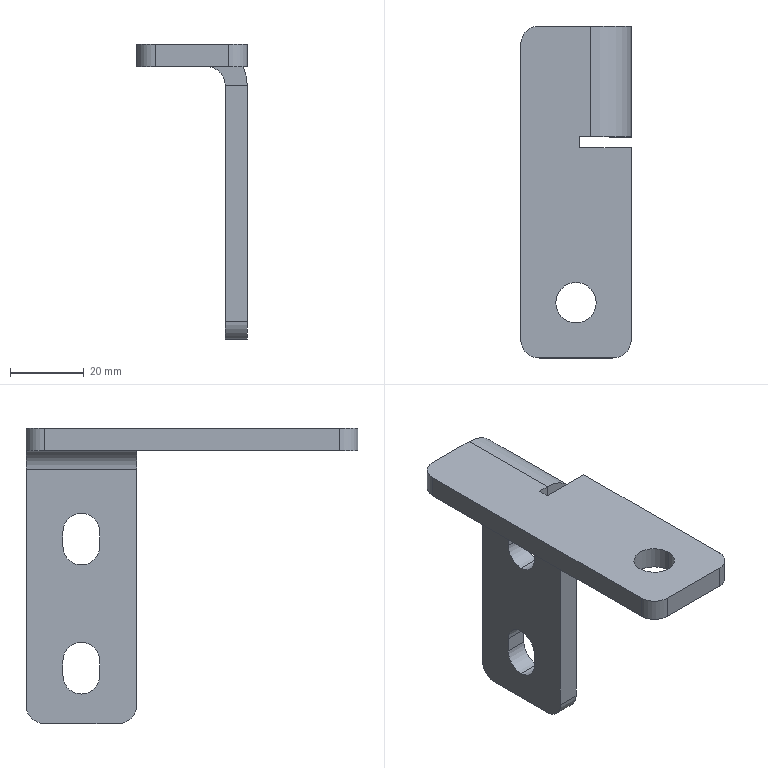Part | STEP file | SYL_0392D6J1SYL0380DJ1006_2_6-5 | 1 solid | 37 faces | box 30 x 90 x 80 mm | volume 26496 mm3 | plane 20 | cylinder 17 | commonest cylinder face diameters 10 x14 11 x2 22 x1
STEP:
#1=CARTESIAN_POINT('',(15.,35.,-61.));
#2=VERTEX_POINT('',#1);
#3=CARTESIAN_POINT('',(9.,35.,-61.));
#4=VERTEX_POINT('',#3);
#5=CARTESIAN_POINT('',(9.,35.,-61.));
#6=DIRECTION('',(-1.,0.,0.));
#7=VECTOR('',#6,1000.);
#8=LINE('',#5,#7);
#9=EDGE_CURVE('',#2,#4,#8,.T.);
#10=ORIENTED_EDGE('',*,*,#9,.F.);
#11=CARTESIAN_POINT('',(15.,35.,-57.));
#12=VERTEX_POINT('',#11);
#13=CARTESIAN_POINT('',(15.,35.,6.));
#14=DIRECTION('',(0.,0.,1.));
#15=VECTOR('',#14,1000.);
#16=LINE('',#13,#15);
#17=EDGE_CURVE('',#2,#12,#16,.T.);
#18=ORIENTED_EDGE('',*,*,#17,.T.);
#19=CARTESIAN_POINT('',(9.,35.,-57.));
#20=VERTEX_POINT('',#19);
#21=CARTESIAN_POINT('',(9.,35.,-57.));
#22=DIRECTION('',(-1.,0.,0.));
#23=VECTOR('',#22,1000.);
#24=LINE('',#21,#23);
#25=EDGE_CURVE('',#12,#20,#24,.T.);
#26=ORIENTED_EDGE('',*,*,#25,.T.);
#27=CARTESIAN_POINT('',(9.,35.,-61.));
#28=DIRECTION('',(0.,0.,1.));
#29=VECTOR('',#28,1000.);
#30=LINE('',#27,#29);
#31=EDGE_CURVE('',#4,#20,#30,.T.);
#32=ORIENTED_EDGE('',*,*,#31,.F.);
#33=EDGE_LOOP('',(#10,#18,#26,#32));
#34=FACE_OUTER_BOUND('',#33,.T.);
#35=CARTESIAN_POINT('',(9.,35.,-61.));
#36=DIRECTION('',(0.,1.,0.));
#37=DIRECTION('',(0.,0.,1.));
#38=AXIS2_PLACEMENT_3D('',#35,#36,#37);
#39=PLANE('',#38);
#40=ADVANCED_FACE('',(#34),#39,.F.);
#41=ORIENTED_EDGE('',*,*,#25,.F.);
#42=CARTESIAN_POINT('',(15.,30.,-52.));
#43=VERTEX_POINT('',#42);
#44=CARTESIAN_POINT('',(15.,30.,-57.));
#45=DIRECTION('',(1.,0.,0.));
#46=DIRECTION('',(0.,0.,-1.));
#47=AXIS2_PLACEMENT_3D('',#44,#45,#46);
#48=CIRCLE('',#47,5.);
#49=EDGE_CURVE('',#12,#43,#48,.T.);
#50=ORIENTED_EDGE('',*,*,#49,.T.);
#51=CARTESIAN_POINT('',(9.,30.,-52.));
#52=VERTEX_POINT('',#51);
#53=CARTESIAN_POINT('',(9.,30.,-52.));
#54=DIRECTION('',(-1.,0.,0.));
#55=VECTOR('',#54,1000.);
#56=LINE('',#53,#55);
#57=EDGE_CURVE('',#43,#52,#56,.T.);
#58=ORIENTED_EDGE('',*,*,#57,.T.);
#59=CARTESIAN_POINT('',(9.,30.,-57.));
#60=DIRECTION('',(1.,0.,0.));
#61=DIRECTION('',(0.,1.,0.));
#62=AXIS2_PLACEMENT_3D('',#59,#60,#61);
#63=CIRCLE('',#62,5.);
#64=EDGE_CURVE('',#20,#52,#63,.T.);
#65=ORIENTED_EDGE('',*,*,#64,.F.);
#66=EDGE_LOOP('',(#41,#50,#58,#65));
#67=FACE_OUTER_BOUND('',#66,.T.);
#68=CARTESIAN_POINT('',(9.,30.,-57.));
#69=DIRECTION('',(1.,0.,0.));
#70=DIRECTION('',(0.,0.,-1.));
#71=AXIS2_PLACEMENT_3D('',#68,#69,#70);
#72=CYLINDRICAL_SURFACE('',#71,5.);
#73=ADVANCED_FACE('',(#67),#72,.F.);
#74=ORIENTED_EDGE('',*,*,#57,.F.);
#75=CARTESIAN_POINT('',(15.,25.,-57.));
#76=VERTEX_POINT('',#75);
#77=CARTESIAN_POINT('',(15.,30.,-57.));
#78=DIRECTION('',(1.,0.,0.));
#79=DIRECTION('',(0.,0.,-1.));
#80=AXIS2_PLACEMENT_3D('',#77,#78,#79);
#81=CIRCLE('',#80,5.);
#82=EDGE_CURVE('',#43,#76,#81,.T.);
#83=ORIENTED_EDGE('',*,*,#82,.T.);
#84=CARTESIAN_POINT('',(9.,25.,-57.));
#85=VERTEX_POINT('',#84);
#86=CARTESIAN_POINT('',(9.,25.,-57.));
#87=DIRECTION('',(-1.,0.,0.));
#88=VECTOR('',#87,1000.);
#89=LINE('',#86,#88);
#90=EDGE_CURVE('',#76,#85,#89,.T.);
#91=ORIENTED_EDGE('',*,*,#90,.T.);
#92=CARTESIAN_POINT('',(9.,30.,-57.));
#93=DIRECTION('',(1.,0.,0.));
#94=DIRECTION('',(0.,0.,1.));
#95=AXIS2_PLACEMENT_3D('',#92,#93,#94);
#96=CIRCLE('',#95,5.);
#97=EDGE_CURVE('',#52,#85,#96,.T.);
#98=ORIENTED_EDGE('',*,*,#97,.F.);
#99=EDGE_LOOP('',(#74,#83,#91,#98));
#100=FACE_OUTER_BOUND('',#99,.T.);
#101=CARTESIAN_POINT('',(9.,30.,-57.));
#102=DIRECTION('',(1.,0.,0.));
#103=DIRECTION('',(0.,0.,-1.));
#104=AXIS2_PLACEMENT_3D('',#101,#102,#103);
#105=CYLINDRICAL_SURFACE('',#104,5.);
#106=ADVANCED_FACE('',(#100),#105,.F.);
#107=ORIENTED_EDGE('',*,*,#90,.F.);
#108=CARTESIAN_POINT('',(15.,25.,-61.));
#109=VERTEX_POINT('',#108);
#110=CARTESIAN_POINT('',(15.,25.,6.));
#111=DIRECTION('',(0.,0.,-1.));
#112=VECTOR('',#111,1000.);
#113=LINE('',#110,#112);
#114=EDGE_CURVE('',#76,#109,#113,.T.);
#115=ORIENTED_EDGE('',*,*,#114,.T.);
#116=CARTESIAN_POINT('',(9.,25.,-61.));
#117=VERTEX_POINT('',#116);
#118=CARTESIAN_POINT('',(9.,25.,-61.));
#119=DIRECTION('',(-1.,0.,0.));
#120=VECTOR('',#119,1000.);
#121=LINE('',#118,#120);
#122=EDGE_CURVE('',#109,#117,#121,.T.);
#123=ORIENTED_EDGE('',*,*,#122,.T.);
#124=CARTESIAN_POINT('',(9.,25.,-57.));
#125=DIRECTION('',(0.,0.,-1.));
#126=VECTOR('',#125,1000.);
#127=LINE('',#124,#126);
#128=EDGE_CURVE('',#85,#117,#127,.T.);
#129=ORIENTED_EDGE('',*,*,#128,.F.);
#130=EDGE_LOOP('',(#107,#115,#123,#129));
#131=FACE_OUTER_BOUND('',#130,.T.);
#132=CARTESIAN_POINT('',(9.,25.,-57.));
#133=DIRECTION('',(0.,-1.,0.));
#134=DIRECTION('',(0.,0.,-1.));
#135=AXIS2_PLACEMENT_3D('',#132,#133,#134);
#136=PLANE('',#135);
#137=ADVANCED_FACE('',(#131),#136,.F.);
#138=ORIENTED_EDGE('',*,*,#122,.F.);
#139=CARTESIAN_POINT('',(15.,30.,-66.));
#140=VERTEX_POINT('',#139);
#141=CARTESIAN_POINT('',(15.,30.,-61.));
#142=DIRECTION('',(1.,0.,0.));
#143=DIRECTION('',(0.,0.,-1.));
#144=AXIS2_PLACEMENT_3D('',#141,#142,#143);
#145=CIRCLE('',#144,5.);
#146=EDGE_CURVE('',#109,#140,#145,.T.);
#147=ORIENTED_EDGE('',*,*,#146,.T.);
#148=CARTESIAN_POINT('',(9.,30.,-66.));
#149=VERTEX_POINT('',#148);
#150=CARTESIAN_POINT('',(9.,30.,-66.));
#151=DIRECTION('',(-1.,0.,0.));
#152=VECTOR('',#151,1000.);
#153=LINE('',#150,#152);
#154=EDGE_CURVE('',#140,#149,#153,.T.);
#155=ORIENTED_EDGE('',*,*,#154,.T.);
#156=CARTESIAN_POINT('',(9.,30.,-61.));
#157=DIRECTION('',(1.,0.,0.));
#158=DIRECTION('',(0.,-1.,0.));
#159=AXIS2_PLACEMENT_3D('',#156,#157,#158);
#160=CIRCLE('',#159,5.);
#161=EDGE_CURVE('',#117,#149,#160,.T.);
#162=ORIENTED_EDGE('',*,*,#161,.F.);
#163=EDGE_LOOP('',(#138,#147,#155,#162));
#164=FACE_OUTER_BOUND('',#163,.T.);
#165=CARTESIAN_POINT('',(9.,30.,-61.));
#166=DIRECTION('',(1.,0.,0.));
#167=DIRECTION('',(0.,0.,-1.));
#168=AXIS2_PLACEMENT_3D('',#165,#166,#167);
#169=CYLINDRICAL_SURFACE('',#168,5.);
#170=ADVANCED_FACE('',(#164),#169,.F.);
#171=CARTESIAN_POINT('',(15.,35.,-26.));
#172=VERTEX_POINT('',#171);
#173=CARTESIAN_POINT('',(9.,35.,-26.));
#174=VERTEX_POINT('',#173);
#175=CARTESIAN_POINT('',(9.,35.,-26.));
#176=DIRECTION('',(-1.,0.,0.));
#177=VECTOR('',#176,1000.);
#178=LINE('',#175,#177);
#179=EDGE_CURVE('',#172,#174,#178,.T.);
#180=ORIENTED_EDGE('',*,*,#179,.F.);
#181=CARTESIAN_POINT('',(15.,35.,-22.));
#182=VERTEX_POINT('',#181);
#183=CARTESIAN_POINT('',(15.,35.,6.));
#184=DIRECTION('',(0.,0.,1.));
#185=VECTOR('',#184,1000.);
#186=LINE('',#183,#185);
#187=EDGE_CURVE('',#172,#182,#186,.T.);
#188=ORIENTED_EDGE('',*,*,#187,.T.);
#189=CARTESIAN_POINT('',(9.,35.,-22.));
#190=VERTEX_POINT('',#189);
#191=CARTESIAN_POINT('',(9.,35.,-22.));
#192=DIRECTION('',(-1.,0.,0.));
#193=VECTOR('',#192,1000.);
#194=LINE('',#191,#193);
#195=EDGE_CURVE('',#182,#190,#194,.T.);
#196=ORIENTED_EDGE('',*,*,#195,.T.);
#197=CARTESIAN_POINT('',(9.,35.,-26.));
#198=DIRECTION('',(0.,0.,1.));
#199=VECTOR('',#198,1000.);
#200=LINE('',#197,#199);
#201=EDGE_CURVE('',#174,#190,#200,.T.);
#202=ORIENTED_EDGE('',*,*,#201,.F.);
#203=EDGE_LOOP('',(#180,#188,#196,#202));
#204=FACE_OUTER_BOUND('',#203,.T.);
#205=CARTESIAN_POINT('',(9.,35.,-26.));
#206=DIRECTION('',(0.,1.,0.));
#207=DIRECTION('',(0.,0.,1.));
#208=AXIS2_PLACEMENT_3D('',#205,#206,#207);
#209=PLANE('',#208);
#210=ADVANCED_FACE('',(#204),#209,.F.);
#211=ORIENTED_EDGE('',*,*,#195,.F.);
#212=CARTESIAN_POINT('',(15.,30.,-17.));
#213=VERTEX_POINT('',#212);
#214=CARTESIAN_POINT('',(15.,30.,-22.));
#215=DIRECTION('',(1.,0.,0.));
#216=DIRECTION('',(0.,0.,-1.));
#217=AXIS2_PLACEMENT_3D('',#214,#215,#216);
#218=CIRCLE('',#217,5.);
#219=EDGE_CURVE('',#182,#213,#218,.T.);
#220=ORIENTED_EDGE('',*,*,#219,.T.);
#221=CARTESIAN_POINT('',(9.,30.,-17.));
#222=VERTEX_POINT('',#221);
#223=CARTESIAN_POINT('',(9.,30.,-17.));
#224=DIRECTION('',(-1.,0.,0.));
#225=VECTOR('',#224,1000.);
#226=LINE('',#223,#225);
#227=EDGE_CURVE('',#213,#222,#226,.T.);
#228=ORIENTED_EDGE('',*,*,#227,.T.);
#229=CARTESIAN_POINT('',(9.,30.,-22.));
#230=DIRECTION('',(1.,0.,0.));
#231=DIRECTION('',(0.,1.,0.));
#232=AXIS2_PLACEMENT_3D('',#229,#230,#231);
#233=CIRCLE('',#232,5.);
#234=EDGE_CURVE('',#190,#222,#233,.T.);
#235=ORIENTED_EDGE('',*,*,#234,.F.);
#236=EDGE_LOOP('',(#211,#220,#228,#235));
#237=FACE_OUTER_BOUND('',#236,.T.);
#238=CARTESIAN_POINT('',(9.,30.,-22.));
#239=DIRECTION('',(1.,0.,0.));
#240=DIRECTION('',(0.,0.,-1.));
#241=AXIS2_PLACEMENT_3D('',#238,#239,#240);
#242=CYLINDRICAL_SURFACE('',#241,5.);
#243=ADVANCED_FACE('',(#237),#242,.F.);
#244=ORIENTED_EDGE('',*,*,#227,.F.);
#245=CARTESIAN_POINT('',(15.,25.,-22.));
#246=VERTEX_POINT('',#245);
#247=CARTESIAN_POINT('',(15.,30.,-22.));
#248=DIRECTION('',(1.,0.,0.));
#249=DIRECTION('',(0.,0.,-1.));
#250=AXIS2_PLACEMENT_3D('',#247,#248,#249);
#251=CIRCLE('',#250,5.);
#252=EDGE_CURVE('',#213,#246,#251,.T.);
#253=ORIENTED_EDGE('',*,*,#252,.T.);
#254=CARTESIAN_POINT('',(9.,25.,-22.));
#255=VERTEX_POINT('',#254);
#256=CARTESIAN_POINT('',(9.,25.,-22.));
#257=DIRECTION('',(-1.,0.,0.));
#258=VECTOR('',#257,1000.);
#259=LINE('',#256,#258);
#260=EDGE_CURVE('',#246,#255,#259,.T.);
#261=ORIENTED_EDGE('',*,*,#260,.T.);
#262=CARTESIAN_POINT('',(9.,30.,-22.));
#263=DIRECTION('',(1.,0.,0.));
#264=DIRECTION('',(0.,0.,1.));
#265=AXIS2_PLACEMENT_3D('',#262,#263,#264);
#266=CIRCLE('',#265,5.);
#267=EDGE_CURVE('',#222,#255,#266,.T.);
#268=ORIENTED_EDGE('',*,*,#267,.F.);
#269=EDGE_LOOP('',(#244,#253,#261,#268));
#270=FACE_OUTER_BOUND('',#269,.T.);
#271=CARTESIAN_POINT('',(9.,30.,-22.));
#272=DIRECTION('',(1.,0.,0.));
#273=DIRECTION('',(0.,0.,-1.));
#274=AXIS2_PLACEMENT_3D('',#271,#272,#273);
#275=CYLINDRICAL_SURFACE('',#274,5.);
#276=ADVANCED_FACE('',(#270),#275,.F.);
#277=ORIENTED_EDGE('',*,*,#260,.F.);
#278=CARTESIAN_POINT('',(15.,25.,-26.));
#279=VERTEX_POINT('',#278);
#280=CARTESIAN_POINT('',(15.,25.,6.));
#281=DIRECTION('',(0.,0.,-1.));
#282=VECTOR('',#281,1000.);
#283=LINE('',#280,#282);
#284=EDGE_CURVE('',#246,#279,#283,.T.);
#285=ORIENTED_EDGE('',*,*,#284,.T.);
#286=CARTESIAN_POINT('',(9.,25.,-26.));
#287=VERTEX_POINT('',#286);
#288=CARTESIAN_POINT('',(9.,25.,-26.));
#289=DIRECTION('',(-1.,0.,0.));
#290=VECTOR('',#289,1000.);
#291=LINE('',#288,#290);
#292=EDGE_CURVE('',#279,#287,#291,.T.);
#293=ORIENTED_EDGE('',*,*,#292,.T.);
#294=CARTESIAN_POINT('',(9.,25.,-22.));
#295=DIRECTION('',(0.,0.,-1.));
#296=VECTOR('',#295,1000.);
#297=LINE('',#294,#296);
#298=EDGE_CURVE('',#255,#287,#297,.T.);
#299=ORIENTED_EDGE('',*,*,#298,.F.);
#300=EDGE_LOOP('',(#277,#285,#293,#299));
#301=FACE_OUTER_BOUND('',#300,.T.);
#302=CARTESIAN_POINT('',(9.,25.,-22.));
#303=DIRECTION('',(0.,-1.,0.));
#304=DIRECTION('',(0.,0.,-1.));
#305=AXIS2_PLACEMENT_3D('',#302,#303,#304);
#306=PLANE('',#305);
#307=ADVANCED_FACE('',(#301),#306,.F.);
#308=ORIENTED_EDGE('',*,*,#292,.F.);
#309=CARTESIAN_POINT('',(15.,30.,-31.));
#310=VERTEX_POINT('',#309);
#311=CARTESIAN_POINT('',(15.,30.,-26.));
#312=DIRECTION('',(1.,0.,0.));
#313=DIRECTION('',(0.,0.,-1.));
#314=AXIS2_PLACEMENT_3D('',#311,#312,#313);
#315=CIRCLE('',#314,5.);
#316=EDGE_CURVE('',#279,#310,#315,.T.);
#317=ORIENTED_EDGE('',*,*,#316,.T.);
#318=CARTESIAN_POINT('',(9.,30.,-31.));
#319=VERTEX_POINT('',#318);
#320=CARTESIAN_POINT('',(9.,30.,-31.));
#321=DIRECTION('',(-1.,0.,0.));
#322=VECTOR('',#321,1000.);
#323=LINE('',#320,#322);
#324=EDGE_CURVE('',#310,#319,#323,.T.);
#325=ORIENTED_EDGE('',*,*,#324,.T.);
#326=CARTESIAN_POINT('',(9.,30.,-26.));
#327=DIRECTION('',(1.,0.,0.));
#328=DIRECTION('',(0.,-1.,0.));
#329=AXIS2_PLACEMENT_3D('',#326,#327,#328);
#330=CIRCLE('',#329,5.);
#331=EDGE_CURVE('',#287,#319,#330,.T.);
#332=ORIENTED_EDGE('',*,*,#331,.F.);
#333=EDGE_LOOP('',(#308,#317,#325,#332));
#334=FACE_OUTER_BOUND('',#333,.T.);
#335=CARTESIAN_POINT('',(9.,30.,-26.));
#336=DIRECTION('',(1.,0.,0.));
#337=DIRECTION('',(0.,0.,-1.));
#338=AXIS2_PLACEMENT_3D('',#335,#336,#337);
#339=CYLINDRICAL_SURFACE('',#338,5.);
#340=ADVANCED_FACE('',(#334),#339,.F.);
#341=CARTESIAN_POINT('',(-5.5,-30.,6.));
#342=VERTEX_POINT('',#341);
#343=CARTESIAN_POINT('',(-5.5,-30.,0.));
#344=VERTEX_POINT('',#343);
#345=CARTESIAN_POINT('',(-5.5,-30.,0.));
#346=DIRECTION('',(0.,0.,-1.));
#347=VECTOR('',#346,1000.);
#348=LINE('',#345,#347);
#349=EDGE_CURVE('',#342,#344,#348,.T.);
#350=ORIENTED_EDGE('',*,*,#349,.F.);
#351=CARTESIAN_POINT('',(5.5,-30.,6.));
#352=VERTEX_POINT('',#351);
#353=CARTESIAN_POINT('',(0.,-30.,6.));
#354=DIRECTION('',(0.,0.,1.));
#355=DIRECTION('',(1.,0.,0.));
#356=AXIS2_PLACEMENT_3D('',#353,#354,#355);
#357=CIRCLE('',#356,5.5);
#358=EDGE_CURVE('',#342,#352,#357,.T.);
#359=ORIENTED_EDGE('',*,*,#358,.T.);
#360=CARTESIAN_POINT('',(5.5,-30.,0.));
#361=VERTEX_POINT('',#360);
#362=CARTESIAN_POINT('',(5.5,-30.,0.));
#363=DIRECTION('',(0.,0.,-1.));
#364=VECTOR('',#363,1000.);
#365=LINE('',#362,#364);
#366=EDGE_CURVE('',#352,#361,#365,.T.);
#367=ORIENTED_EDGE('',*,*,#366,.T.);
#368=CARTESIAN_POINT('',(0.,-30.,0.));
#369=DIRECTION('',(0.,0.,1.));
#370=DIRECTION('',(-1.,0.,0.));
#371=AXIS2_PLACEMENT_3D('',#368,#369,#370);
#372=CIRCLE('',#371,5.5);
#373=EDGE_CURVE('',#344,#361,#372,.T.);
#374=ORIENTED_EDGE('',*,*,#373,.F.);
#375=EDGE_LOOP('',(#350,#359,#367,#374));
#376=FACE_OUTER_BOUND('',#375,.T.);
#377=CARTESIAN_POINT('',(0.,-30.,0.));
#378=DIRECTION('',(0.,0.,1.));
#379=DIRECTION('',(1.,0.,0.));
#380=AXIS2_PLACEMENT_3D('',#377,#378,#379);
#381=CYLINDRICAL_SURFACE('',#380,5.5);
#382=ADVANCED_FACE('',(#376),#381,.F.);
#383=CARTESIAN_POINT('',(15.,45.,-69.));
#384=VERTEX_POINT('',#383);
#385=CARTESIAN_POINT('',(9.,45.,-69.));
#386=VERTEX_POINT('',#385);
#387=CARTESIAN_POINT('',(9.,45.,-69.));
#388=DIRECTION('',(-1.,0.,0.));
#389=VECTOR('',#388,1000.);
#390=LINE('',#387,#389);
#391=EDGE_CURVE('',#384,#386,#390,.T.);
#392=ORIENTED_EDGE('',*,*,#391,.F.);
#393=CARTESIAN_POINT('',(15.,40.,-74.));
#394=VERTEX_POINT('',#393);
#395=CARTESIAN_POINT('',(15.,40.,-69.));
#396=DIRECTION('',(-1.,0.,0.));
#397=DIRECTION('',(0.,0.,1.));
#398=AXIS2_PLACEMENT_3D('',#395,#396,#397);
#399=CIRCLE('',#398,5.);
#400=EDGE_CURVE('',#384,#394,#399,.T.);
#401=ORIENTED_EDGE('',*,*,#400,.T.);
#402=CARTESIAN_POINT('',(9.,40.,-74.));
#403=VERTEX_POINT('',#402);
#404=CARTESIAN_POINT('',(9.,40.,-74.));
#405=DIRECTION('',(-1.,0.,0.));
#406=VECTOR('',#405,1000.);
#407=LINE('',#404,#406);
#408=EDGE_CURVE('',#394,#403,#407,.T.);
#409=ORIENTED_EDGE('',*,*,#408,.T.);
#410=CARTESIAN_POINT('',(9.,40.,-69.));
#411=DIRECTION('',(-1.,0.,0.));
#412=DIRECTION('',(0.,1.,0.));
#413=AXIS2_PLACEMENT_3D('',#410,#411,#412);
#414=CIRCLE('',#413,5.);
#415=EDGE_CURVE('',#386,#403,#414,.T.);
#416=ORIENTED_EDGE('',*,*,#415,.F.);
#417=EDGE_LOOP('',(#392,#401,#409,#416));
#418=FACE_OUTER_BOUND('',#417,.T.);
#419=CARTESIAN_POINT('',(9.,40.,-69.));
#420=DIRECTION('',(1.,0.,0.));
#421=DIRECTION('',(0.,0.,-1.));
#422=AXIS2_PLACEMENT_3D('',#419,#420,#421);
#423=CYLINDRICAL_SURFACE('',#422,5.);
#424=ADVANCED_FACE('',(#418),#423,.T.);
#425=ORIENTED_EDGE('',*,*,#408,.F.);
#426=CARTESIAN_POINT('',(15.,20.,-74.));
#427=VERTEX_POINT('',#426);
#428=CARTESIAN_POINT('',(15.,-23.616,-74.));
#429=DIRECTION('',(0.,-1.,0.));
#430=VECTOR('',#429,1000.);
#431=LINE('',#428,#430);
#432=EDGE_CURVE('',#394,#427,#431,.T.);
#433=ORIENTED_EDGE('',*,*,#432,.T.);
#434=CARTESIAN_POINT('',(9.,20.,-74.));
#435=VERTEX_POINT('',#434);
#436=CARTESIAN_POINT('',(9.,20.,-74.));
#437=DIRECTION('',(-1.,0.,0.));
#438=VECTOR('',#437,1000.);
#439=LINE('',#436,#438);
#440=EDGE_CURVE('',#427,#435,#439,.T.);
#441=ORIENTED_EDGE('',*,*,#440,.T.);
#442=CARTESIAN_POINT('',(9.,40.,-74.));
#443=DIRECTION('',(0.,-1.,0.));
#444=VECTOR('',#443,1000.);
#445=LINE('',#442,#444);
#446=EDGE_CURVE('',#403,#435,#445,.T.);
#447=ORIENTED_EDGE('',*,*,#446,.F.);
#448=EDGE_LOOP('',(#425,#433,#441,#447));
#449=FACE_OUTER_BOUND('',#448,.T.);
#450=CARTESIAN_POINT('',(9.,40.,-74.));
#451=DIRECTION('',(0.,0.,1.));
#452=DIRECTION('',(0.,-1.,0.));
#453=AXIS2_PLACEMENT_3D('',#450,#451,#452);
#454=PLANE('',#453);
#455=ADVANCED_FACE('',(#449),#454,.F.);
#456=ORIENTED_EDGE('',*,*,#440,.F.);
#457=CARTESIAN_POINT('',(15.,15.,-69.));
#458=VERTEX_POINT('',#457);
#459=CARTESIAN_POINT('',(15.,20.,-69.));
#460=DIRECTION('',(-1.,0.,0.));
#461=DIRECTION('',(0.,0.,1.));
#462=AXIS2_PLACEMENT_3D('',#459,#460,#461);
#463=CIRCLE('',#462,5.);
#464=EDGE_CURVE('',#427,#458,#463,.T.);
#465=ORIENTED_EDGE('',*,*,#464,.T.);
#466=CARTESIAN_POINT('',(9.,15.,-69.));
#467=VERTEX_POINT('',#466);
#468=CARTESIAN_POINT('',(9.,15.,-69.));
#469=DIRECTION('',(-1.,0.,0.));
#470=VECTOR('',#469,1000.);
#471=LINE('',#468,#470);
#472=EDGE_CURVE('',#458,#467,#471,.T.);
#473=ORIENTED_EDGE('',*,*,#472,.T.);
#474=CARTESIAN_POINT('',(9.,20.,-69.));
#475=DIRECTION('',(-1.,0.,0.));
#476=DIRECTION('',(0.,0.,-1.));
#477=AXIS2_PLACEMENT_3D('',#474,#475,#476);
#478=CIRCLE('',#477,5.);
#479=EDGE_CURVE('',#435,#467,#478,.T.);
#480=ORIENTED_EDGE('',*,*,#479,.F.);
#481=EDGE_LOOP('',(#456,#465,#473,#480));
#482=FACE_OUTER_BOUND('',#481,.T.);
#483=CARTESIAN_POINT('',(9.,20.,-69.));
#484=DIRECTION('',(1.,0.,0.));
#485=DIRECTION('',(0.,0.,-1.));
#486=AXIS2_PLACEMENT_3D('',#483,#484,#485);
#487=CYLINDRICAL_SURFACE('',#486,5.);
#488=ADVANCED_FACE('',(#482),#487,.T.);
#489=ORIENTED_EDGE('',*,*,#472,.F.);
#490=CARTESIAN_POINT('',(15.,15.,-5.));
#491=VERTEX_POINT('',#490);
#492=CARTESIAN_POINT('',(15.,15.,6.));
#493=DIRECTION('',(0.,0.,1.));
#494=VECTOR('',#493,1000.);
#495=LINE('',#492,#494);
#496=EDGE_CURVE('',#458,#491,#495,.T.);
#497=ORIENTED_EDGE('',*,*,#496,.T.);
#498=CARTESIAN_POINT('',(9.,15.,-5.));
#499=VERTEX_POINT('',#498);
#500=CARTESIAN_POINT('',(9.,15.,-5.));
#501=DIRECTION('',(-1.,0.,0.));
#502=VECTOR('',#501,1000.);
#503=LINE('',#500,#502);
#504=EDGE_CURVE('',#491,#499,#503,.T.);
#505=ORIENTED_EDGE('',*,*,#504,.T.);
#506=CARTESIAN_POINT('',(9.,15.,-69.));
#507=DIRECTION('',(0.,0.,1.));
#508=VECTOR('',#507,1000.);
#509=LINE('',#506,#508);
#510=EDGE_CURVE('',#467,#499,#509,.T.);
#511=ORIENTED_EDGE('',*,*,#510,.F.);
#512=EDGE_LOOP('',(#489,#497,#505,#511));
#513=FACE_OUTER_BOUND('',#512,.T.);
#514=CARTESIAN_POINT('',(9.,15.,-69.));
#515=DIRECTION('',(0.,1.,0.));
#516=DIRECTION('',(0.,0.,1.));
#517=AXIS2_PLACEMENT_3D('',#514,#515,#516);
#518=PLANE('',#517);
#519=ADVANCED_FACE('',(#513),#518,.F.);
#520=ORIENTED_EDGE('',*,*,#504,.F.);
#521=CARTESIAN_POINT('',(4.,15.,6.));
#522=VERTEX_POINT('',#521);
#523=CARTESIAN_POINT('',(4.,15.,-5.));
#524=DIRECTION('',(0.,1.,0.));
#525=DIRECTION('',(0.,0.,-1.));
#526=AXIS2_PLACEMENT_3D('',#523,#524,#525);
#527=CIRCLE('',#526,11.);
#528=EDGE_CURVE('',#522,#491,#527,.T.);
#529=ORIENTED_EDGE('',*,*,#528,.F.);
#530=CARTESIAN_POINT('',(4.,15.,0.));
#531=VERTEX_POINT('',#530);
#532=CARTESIAN_POINT('',(4.,15.,0.));
#533=DIRECTION('',(0.,0.,-1.));
#534=VECTOR('',#533,1000.);
#535=LINE('',#532,#534);
#536=EDGE_CURVE('',#522,#531,#535,.T.);
#537=ORIENTED_EDGE('',*,*,#536,.T.);
#538=CARTESIAN_POINT('',(4.,15.,-5.));
#539=DIRECTION('',(0.,1.,0.));
#540=DIRECTION('',(0.,0.,1.));
#541=AXIS2_PLACEMENT_3D('',#538,#539,#540);
#542=CIRCLE('',#541,5.);
#543=EDGE_CURVE('',#531,#499,#542,.T.);
#544=ORIENTED_EDGE('',*,*,#543,.T.);
#545=EDGE_LOOP('',(#520,#529,#537,#544));
#546=FACE_OUTER_BOUND('',#545,.T.);
#547=CARTESIAN_POINT('',(4.,15.,-5.));
#548=DIRECTION('',(0.,-1.,0.));
#549=DIRECTION('',(0.,0.,-1.));
#550=AXIS2_PLACEMENT_3D('',#547,#548,#549);
#551=PLANE('',#550);
#552=ADVANCED_FACE('',(#546),#551,.T.);
#553=ORIENTED_EDGE('',*,*,#536,.F.);
#554=CARTESIAN_POINT('',(1.,15.,6.));
#555=VERTEX_POINT('',#554);
#556=CARTESIAN_POINT('',(0.,15.,6.));
#557=DIRECTION('',(-1.,0.,0.));
#558=VECTOR('',#557,1000.);
#559=LINE('',#556,#558);
#560=EDGE_CURVE('',#522,#555,#559,.T.);
#561=ORIENTED_EDGE('',*,*,#560,.T.);
#562=CARTESIAN_POINT('',(1.,15.,0.));
#563=VERTEX_POINT('',#562);
#564=CARTESIAN_POINT('',(1.,15.,0.));
#565=DIRECTION('',(0.,0.,-1.));
#566=VECTOR('',#565,1000.);
#567=LINE('',#564,#566);
#568=EDGE_CURVE('',#555,#563,#567,.T.);
#569=ORIENTED_EDGE('',*,*,#568,.T.);
#570=CARTESIAN_POINT('',(0.,15.,0.));
#571=DIRECTION('',(-1.,0.,0.));
#572=VECTOR('',#571,1000.);
#573=LINE('',#570,#572);
#574=EDGE_CURVE('',#531,#563,#573,.T.);
#575=ORIENTED_EDGE('',*,*,#574,.F.);
#576=EDGE_LOOP('',(#553,#561,#569,#575));
#577=FACE_OUTER_BOUND('',#576,.T.);
#578=CARTESIAN_POINT('',(0.,15.,0.));
#579=DIRECTION('',(0.,1.,0.));
#580=DIRECTION('',(-1.,0.,0.));
#581=AXIS2_PLACEMENT_3D('',#578,#579,#580);
#582=PLANE('',#581);
#583=ADVANCED_FACE('',(#577),#582,.F.);
#584=ORIENTED_EDGE('',*,*,#568,.F.);
#585=CARTESIAN_POINT('',(1.,12.,6.));
#586=VERTEX_POINT('',#585);
#587=CARTESIAN_POINT('',(1.,0.,6.));
#588=DIRECTION('',(0.,-1.,0.));
#589=VECTOR('',#588,1000.);
#590=LINE('',#587,#589);
#591=EDGE_CURVE('',#555,#586,#590,.T.);
#592=ORIENTED_EDGE('',*,*,#591,.T.);
#593=CARTESIAN_POINT('',(1.,12.,0.));
#594=VERTEX_POINT('',#593);
#595=CARTESIAN_POINT('',(1.,12.,0.));
#596=DIRECTION('',(0.,0.,-1.));
#597=VECTOR('',#596,1000.);
#598=LINE('',#595,#597);
#599=EDGE_CURVE('',#586,#594,#598,.T.);
#600=ORIENTED_EDGE('',*,*,#599,.T.);
#601=CARTESIAN_POINT('',(1.,0.,0.));
#602=DIRECTION('',(0.,-1.,0.));
#603=VECTOR('',#602,1000.);
#604=LINE('',#601,#603);
#605=EDGE_CURVE('',#563,#594,#604,.T.);
#606=ORIENTED_EDGE('',*,*,#605,.F.);
#607=EDGE_LOOP('',(#584,#592,#600,#606));
#608=FACE_OUTER_BOUND('',#607,.T.);
#609=CARTESIAN_POINT('',(1.,0.,0.));
#610=DIRECTION('',(-1.,0.,0.));
#611=DIRECTION('',(0.,-1.,0.));
#612=AXIS2_PLACEMENT_3D('',#609,#610,#611);
#613=PLANE('',#612);
#614=ADVANCED_FACE('',(#608),#613,.F.);
#615=ORIENTED_EDGE('',*,*,#599,.F.);
#616=CARTESIAN_POINT('',(15.,12.,6.));
#617=VERTEX_POINT('',#616);
#618=CARTESIAN_POINT('',(0.,12.,6.));
#619=DIRECTION('',(1.,0.,0.));
#620=VECTOR('',#619,1000.);
#621=LINE('',#618,#620);
#622=EDGE_CURVE('',#586,#617,#621,.T.);
#623=ORIENTED_EDGE('',*,*,#622,.T.);
#624=CARTESIAN_POINT('',(15.,12.,0.));
#625=VERTEX_POINT('',#624);
#626=CARTESIAN_POINT('',(15.,12.,0.));
#627=DIRECTION('',(0.,0.,-1.));
#628=VECTOR('',#627,1000.);
#629=LINE('',#626,#628);
#630=EDGE_CURVE('',#617,#625,#629,.T.);
#631=ORIENTED_EDGE('',*,*,#630,.T.);
#632=CARTESIAN_POINT('',(0.,12.,0.));
#633=DIRECTION('',(1.,0.,0.));
#634=VECTOR('',#633,1000.);
#635=LINE('',#632,#634);
#636=EDGE_CURVE('',#594,#625,#635,.T.);
#637=ORIENTED_EDGE('',*,*,#636,.F.);
#638=EDGE_LOOP('',(#615,#623,#631,#637));
#639=FACE_OUTER_BOUND('',#638,.T.);
#640=CARTESIAN_POINT('',(0.,12.,0.));
#641=DIRECTION('',(0.,-1.,0.));
#642=DIRECTION('',(1.,0.,0.));
#643=AXIS2_PLACEMENT_3D('',#640,#641,#642);
#644=PLANE('',#643);
#645=ADVANCED_FACE('',(#639),#644,.F.);
#646=ORIENTED_EDGE('',*,*,#630,.F.);
#647=CARTESIAN_POINT('',(15.,-40.,6.));
#648=VERTEX_POINT('',#647);
#649=CARTESIAN_POINT('',(15.,0.,6.));
#650=DIRECTION('',(0.,-1.,0.));
#651=VECTOR('',#650,1000.);
#652=LINE('',#649,#651);
#653=EDGE_CURVE('',#617,#648,#652,.T.);
#654=ORIENTED_EDGE('',*,*,#653,.T.);
#655=CARTESIAN_POINT('',(15.,-40.,0.));
#656=VERTEX_POINT('',#655);
#657=CARTESIAN_POINT('',(15.,-40.,0.));
#658=DIRECTION('',(0.,0.,-1.));
#659=VECTOR('',#658,1000.);
#660=LINE('',#657,#659);
#661=EDGE_CURVE('',#648,#656,#660,.T.);
#662=ORIENTED_EDGE('',*,*,#661,.T.);
#663=CARTESIAN_POINT('',(15.,15.,0.));
#664=DIRECTION('',(0.,-1.,0.));
#665=VECTOR('',#664,1000.);
#666=LINE('',#663,#665);
#667=EDGE_CURVE('',#625,#656,#666,.T.);
#668=ORIENTED_EDGE('',*,*,#667,.F.);
#669=EDGE_LOOP('',(#646,#654,#662,#668));
#670=FACE_OUTER_BOUND('',#669,.T.);
#671=CARTESIAN_POINT('',(15.,15.,0.));
#672=DIRECTION('',(-1.,0.,0.));
#673=DIRECTION('',(0.,-1.,0.));
#674=AXIS2_PLACEMENT_3D('',#671,#672,#673);
#675=PLANE('',#674);
#676=ADVANCED_FACE('',(#670),#675,.F.);
#677=ORIENTED_EDGE('',*,*,#661,.F.);
#678=CARTESIAN_POINT('',(10.,-45.,6.));
#679=VERTEX_POINT('',#678);
#680=CARTESIAN_POINT('',(10.,-40.,6.));
#681=DIRECTION('',(0.,0.,-1.));
#682=DIRECTION('',(-1.,0.,0.));
#683=AXIS2_PLACEMENT_3D('',#680,#681,#682);
#684=CIRCLE('',#683,5.);
#685=EDGE_CURVE('',#648,#679,#684,.T.);
#686=ORIENTED_EDGE('',*,*,#685,.T.);
#687=CARTESIAN_POINT('',(10.,-45.,0.));
#688=VERTEX_POINT('',#687);
#689=CARTESIAN_POINT('',(10.,-45.,0.));
#690=DIRECTION('',(0.,0.,-1.));
#691=VECTOR('',#690,1000.);
#692=LINE('',#689,#691);
#693=EDGE_CURVE('',#679,#688,#692,.T.);
#694=ORIENTED_EDGE('',*,*,#693,.T.);
#695=CARTESIAN_POINT('',(10.,-40.,0.));
#696=DIRECTION('',(0.,0.,-1.));
#697=DIRECTION('',(1.,0.,0.));
#698=AXIS2_PLACEMENT_3D('',#695,#696,#697);
#699=CIRCLE('',#698,5.);
#700=EDGE_CURVE('',#656,#688,#699,.T.);
#701=ORIENTED_EDGE('',*,*,#700,.F.);
#702=EDGE_LOOP('',(#677,#686,#694,#701));
#703=FACE_OUTER_BOUND('',#702,.T.);
#704=CARTESIAN_POINT('',(10.,-40.,0.));
#705=DIRECTION('',(0.,0.,1.));
#706=DIRECTION('',(1.,0.,0.));
#707=AXIS2_PLACEMENT_3D('',#704,#705,#706);
#708=CYLINDRICAL_SURFACE('',#707,5.);
#709=ADVANCED_FACE('',(#703),#708,.T.);
#710=ORIENTED_EDGE('',*,*,#693,.F.);
#711=CARTESIAN_POINT('',(-10.,-45.,6.));
#712=VERTEX_POINT('',#711);
#713=CARTESIAN_POINT('',(0.,-45.,6.));
#714=DIRECTION('',(-1.,0.,0.));
#715=VECTOR('',#714,1000.);
#716=LINE('',#713,#715);
#717=EDGE_CURVE('',#679,#712,#716,.T.);
#718=ORIENTED_EDGE('',*,*,#717,.T.);
#719=CARTESIAN_POINT('',(-10.,-45.,0.));
#720=VERTEX_POINT('',#719);
#721=CARTESIAN_POINT('',(-10.,-45.,0.));
#722=DIRECTION('',(0.,0.,-1.));
#723=VECTOR('',#722,1000.);
#724=LINE('',#721,#723);
#725=EDGE_CURVE('',#712,#720,#724,.T.);
#726=ORIENTED_EDGE('',*,*,#725,.T.);
#727=CARTESIAN_POINT('',(10.,-45.,0.));
#728=DIRECTION('',(-1.,0.,0.));
#729=VECTOR('',#728,1000.);
#730=LINE('',#727,#729);
#731=EDGE_CURVE('',#688,#720,#730,.T.);
#732=ORIENTED_EDGE('',*,*,#731,.F.);
#733=EDGE_LOOP('',(#710,#718,#726,#732));
#734=FACE_OUTER_BOUND('',#733,.T.);
#735=CARTESIAN_POINT('',(10.,-45.,0.));
#736=DIRECTION('',(0.,1.,0.));
#737=DIRECTION('',(-1.,0.,0.));
#738=AXIS2_PLACEMENT_3D('',#735,#736,#737);
#739=PLANE('',#738);
#740=ADVANCED_FACE('',(#734),#739,.F.);
#741=ORIENTED_EDGE('',*,*,#725,.F.);
#742=CARTESIAN_POINT('',(-15.,-40.,6.));
#743=VERTEX_POINT('',#742);
#744=CARTESIAN_POINT('',(-10.,-40.,6.));
#745=DIRECTION('',(0.,0.,-1.));
#746=DIRECTION('',(-1.,0.,0.));
#747=AXIS2_PLACEMENT_3D('',#744,#745,#746);
#748=CIRCLE('',#747,5.);
#749=EDGE_CURVE('',#712,#743,#748,.T.);
#750=ORIENTED_EDGE('',*,*,#749,.T.);
#751=CARTESIAN_POINT('',(-15.,-40.,0.));
#752=VERTEX_POINT('',#751);
#753=CARTESIAN_POINT('',(-15.,-40.,0.));
#754=DIRECTION('',(0.,0.,-1.));
#755=VECTOR('',#754,1000.);
#756=LINE('',#753,#755);
#757=EDGE_CURVE('',#743,#752,#756,.T.);
#758=ORIENTED_EDGE('',*,*,#757,.T.);
#759=CARTESIAN_POINT('',(-10.,-40.,0.));
#760=DIRECTION('',(0.,0.,-1.));
#761=DIRECTION('',(0.,-1.,0.));
#762=AXIS2_PLACEMENT_3D('',#759,#760,#761);
#763=CIRCLE('',#762,5.);
#764=EDGE_CURVE('',#720,#752,#763,.T.);
#765=ORIENTED_EDGE('',*,*,#764,.F.);
#766=EDGE_LOOP('',(#741,#750,#758,#765));
#767=FACE_OUTER_BOUND('',#766,.T.);
#768=CARTESIAN_POINT('',(-10.,-40.,0.));
#769=DIRECTION('',(0.,0.,1.));
#770=DIRECTION('',(1.,0.,0.));
#771=AXIS2_PLACEMENT_3D('',#768,#769,#770);
#772=CYLINDRICAL_SURFACE('',#771,5.);
#773=ADVANCED_FACE('',(#767),#772,.T.);
#774=ORIENTED_EDGE('',*,*,#757,.F.);
#775=CARTESIAN_POINT('',(-15.,40.,6.));
#776=VERTEX_POINT('',#775);
#777=CARTESIAN_POINT('',(-15.,0.,6.));
#778=DIRECTION('',(0.,1.,0.));
#779=VECTOR('',#778,1000.);
#780=LINE('',#777,#779);
#781=EDGE_CURVE('',#743,#776,#780,.T.);
#782=ORIENTED_EDGE('',*,*,#781,.T.);
#783=CARTESIAN_POINT('',(-15.,40.,0.));
#784=VERTEX_POINT('',#783);
#785=CARTESIAN_POINT('',(-15.,40.,0.));
#786=DIRECTION('',(0.,0.,-1.));
#787=VECTOR('',#786,1000.);
#788=LINE('',#785,#787);
#789=EDGE_CURVE('',#776,#784,#788,.T.);
#790=ORIENTED_EDGE('',*,*,#789,.T.);
#791=CARTESIAN_POINT('',(-15.,-40.,0.));
#792=DIRECTION('',(0.,1.,0.));
#793=VECTOR('',#792,1000.);
#794=LINE('',#791,#793);
#795=EDGE_CURVE('',#752,#784,#794,.T.);
#796=ORIENTED_EDGE('',*,*,#795,.F.);
#797=EDGE_LOOP('',(#774,#782,#790,#796));
#798=FACE_OUTER_BOUND('',#797,.T.);
#799=CARTESIAN_POINT('',(-15.,-40.,0.));
#800=DIRECTION('',(1.,0.,0.));
#801=DIRECTION('',(0.,1.,0.));
#802=AXIS2_PLACEMENT_3D('',#799,#800,#801);
#803=PLANE('',#802);
#804=ADVANCED_FACE('',(#798),#803,.F.);
#805=ORIENTED_EDGE('',*,*,#789,.F.);
#806=CARTESIAN_POINT('',(-10.,45.,6.));
#807=VERTEX_POINT('',#806);
#808=CARTESIAN_POINT('',(-10.,40.,6.));
#809=DIRECTION('',(0.,0.,-1.));
#810=DIRECTION('',(-1.,0.,0.));
#811=AXIS2_PLACEMENT_3D('',#808,#809,#810);
#812=CIRCLE('',#811,5.);
#813=EDGE_CURVE('',#776,#807,#812,.T.);
#814=ORIENTED_EDGE('',*,*,#813,.T.);
#815=CARTESIAN_POINT('',(-10.,45.,0.));
#816=VERTEX_POINT('',#815);
#817=CARTESIAN_POINT('',(-10.,45.,0.));
#818=DIRECTION('',(0.,0.,-1.));
#819=VECTOR('',#818,1000.);
#820=LINE('',#817,#819);
#821=EDGE_CURVE('',#807,#816,#820,.T.);
#822=ORIENTED_EDGE('',*,*,#821,.T.);
#823=CARTESIAN_POINT('',(-10.,40.,0.));
#824=DIRECTION('',(0.,0.,-1.));
#825=DIRECTION('',(-1.,0.,0.));
#826=AXIS2_PLACEMENT_3D('',#823,#824,#825);
#827=CIRCLE('',#826,5.);
#828=EDGE_CURVE('',#784,#816,#827,.T.);
#829=ORIENTED_EDGE('',*,*,#828,.F.);
#830=EDGE_LOOP('',(#805,#814,#822,#829));
#831=FACE_OUTER_BOUND('',#830,.T.);
#832=CARTESIAN_POINT('',(-10.,40.,0.));
#833=DIRECTION('',(0.,0.,1.));
#834=DIRECTION('',(1.,0.,0.));
#835=AXIS2_PLACEMENT_3D('',#832,#833,#834);
#836=CYLINDRICAL_SURFACE('',#835,5.);
#837=ADVANCED_FACE('',(#831),#836,.T.);
#838=ORIENTED_EDGE('',*,*,#821,.F.);
#839=CARTESIAN_POINT('',(4.,45.,6.));
#840=VERTEX_POINT('',#839);
#841=CARTESIAN_POINT('',(0.,45.,6.));
#842=DIRECTION('',(1.,0.,0.));
#843=VECTOR('',#842,1000.);
#844=LINE('',#841,#843);
#845=EDGE_CURVE('',#807,#840,#844,.T.);
#846=ORIENTED_EDGE('',*,*,#845,.T.);
#847=CARTESIAN_POINT('',(4.,45.,0.));
#848=VERTEX_POINT('',#847);
#849=CARTESIAN_POINT('',(4.,45.,0.));
#850=DIRECTION('',(0.,0.,-1.));
#851=VECTOR('',#850,1000.);
#852=LINE('',#849,#851);
#853=EDGE_CURVE('',#840,#848,#852,.T.);
#854=ORIENTED_EDGE('',*,*,#853,.T.);
#855=CARTESIAN_POINT('',(-10.,45.,0.));
#856=DIRECTION('',(1.,0.,0.));
#857=VECTOR('',#856,1000.);
#858=LINE('',#855,#857);
#859=EDGE_CURVE('',#816,#848,#858,.T.);
#860=ORIENTED_EDGE('',*,*,#859,.F.);
#861=EDGE_LOOP('',(#838,#846,#854,#860));
#862=FACE_OUTER_BOUND('',#861,.T.);
#863=CARTESIAN_POINT('',(-10.,45.,0.));
#864=DIRECTION('',(0.,-1.,0.));
#865=DIRECTION('',(1.,0.,0.));
#866=AXIS2_PLACEMENT_3D('',#863,#864,#865);
#867=PLANE('',#866);
#868=ADVANCED_FACE('',(#862),#867,.F.);
#869=ORIENTED_EDGE('',*,*,#853,.F.);
#870=CARTESIAN_POINT('',(15.,45.,-5.));
#871=VERTEX_POINT('',#870);
#872=CARTESIAN_POINT('',(4.,45.,-5.));
#873=DIRECTION('',(0.,-1.,0.));
#874=DIRECTION('',(0.,0.,-1.));
#875=AXIS2_PLACEMENT_3D('',#872,#873,#874);
#876=CIRCLE('',#875,11.);
#877=EDGE_CURVE('',#871,#840,#876,.T.);
#878=ORIENTED_EDGE('',*,*,#877,.F.);
#879=CARTESIAN_POINT('',(9.,45.,-5.));
#880=VERTEX_POINT('',#879);
#881=CARTESIAN_POINT('',(9.,45.,-5.));
#882=DIRECTION('',(-1.,0.,0.));
#883=VECTOR('',#882,1000.);
#884=LINE('',#881,#883);
#885=EDGE_CURVE('',#871,#880,#884,.T.);
#886=ORIENTED_EDGE('',*,*,#885,.T.);
#887=CARTESIAN_POINT('',(4.,45.,-5.));
#888=DIRECTION('',(0.,-1.,0.));
#889=DIRECTION('',(1.,0.,0.));
#890=AXIS2_PLACEMENT_3D('',#887,#888,#889);
#891=CIRCLE('',#890,5.);
#892=EDGE_CURVE('',#880,#848,#891,.T.);
#893=ORIENTED_EDGE('',*,*,#892,.T.);
#894=EDGE_LOOP('',(#869,#878,#886,#893));
#895=FACE_OUTER_BOUND('',#894,.T.);
#896=CARTESIAN_POINT('',(4.,45.,-5.));
#897=DIRECTION('',(0.,1.,0.));
#898=DIRECTION('',(0.,0.,1.));
#899=AXIS2_PLACEMENT_3D('',#896,#897,#898);
#900=PLANE('',#899);
#901=ADVANCED_FACE('',(#895),#900,.T.);
#902=CARTESIAN_POINT('',(15.,30.,-26.));
#903=DIRECTION('',(1.,0.,0.));
#904=DIRECTION('',(0.,0.,-1.));
#905=AXIS2_PLACEMENT_3D('',#902,#903,#904);
#906=CIRCLE('',#905,5.);
#907=EDGE_CURVE('',#310,#172,#906,.T.);
#908=ORIENTED_EDGE('',*,*,#907,.T.);
#909=ORIENTED_EDGE('',*,*,#179,.T.);
#910=CARTESIAN_POINT('',(9.,30.,-26.));
#911=DIRECTION('',(1.,0.,0.));
#912=DIRECTION('',(0.,0.,-1.));
#913=AXIS2_PLACEMENT_3D('',#910,#911,#912);
#914=CIRCLE('',#913,5.);
#915=EDGE_CURVE('',#319,#174,#914,.T.);
#916=ORIENTED_EDGE('',*,*,#915,.F.);
#917=ORIENTED_EDGE('',*,*,#324,.F.);
#918=EDGE_LOOP('',(#908,#909,#916,#917));
#919=FACE_OUTER_BOUND('',#918,.T.);
#920=CARTESIAN_POINT('',(9.,30.,-26.));
#921=DIRECTION('',(1.,0.,0.));
#922=DIRECTION('',(0.,0.,-1.));
#923=AXIS2_PLACEMENT_3D('',#920,#921,#922);
#924=CYLINDRICAL_SURFACE('',#923,5.);
#925=ADVANCED_FACE('',(#919),#924,.F.);
#926=CARTESIAN_POINT('',(15.,30.,-61.));
#927=DIRECTION('',(1.,0.,0.));
#928=DIRECTION('',(0.,0.,-1.));
#929=AXIS2_PLACEMENT_3D('',#926,#927,#928);
#930=CIRCLE('',#929,5.);
#931=EDGE_CURVE('',#140,#2,#930,.T.);
#932=ORIENTED_EDGE('',*,*,#931,.T.);
#933=ORIENTED_EDGE('',*,*,#9,.T.);
#934=CARTESIAN_POINT('',(9.,30.,-61.));
#935=DIRECTION('',(1.,0.,0.));
#936=DIRECTION('',(0.,0.,-1.));
#937=AXIS2_PLACEMENT_3D('',#934,#935,#936);
#938=CIRCLE('',#937,5.);
#939=EDGE_CURVE('',#149,#4,#938,.T.);
#940=ORIENTED_EDGE('',*,*,#939,.F.);
#941=ORIENTED_EDGE('',*,*,#154,.F.);
#942=EDGE_LOOP('',(#932,#933,#940,#941));
#943=FACE_OUTER_BOUND('',#942,.T.);
#944=CARTESIAN_POINT('',(9.,30.,-61.));
#945=DIRECTION('',(1.,0.,0.));
#946=DIRECTION('',(0.,0.,-1.));
#947=AXIS2_PLACEMENT_3D('',#944,#945,#946);
#948=CYLINDRICAL_SURFACE('',#947,5.);
#949=ADVANCED_FACE('',(#943),#948,.F.);
#950=CARTESIAN_POINT('',(0.,-30.,6.));
#951=DIRECTION('',(0.,0.,1.));
#952=DIRECTION('',(1.,0.,0.));
#953=AXIS2_PLACEMENT_3D('',#950,#951,#952);
#954=CIRCLE('',#953,5.5);
#955=EDGE_CURVE('',#352,#342,#954,.T.);
#956=ORIENTED_EDGE('',*,*,#955,.T.);
#957=ORIENTED_EDGE('',*,*,#349,.T.);
#958=CARTESIAN_POINT('',(0.,-30.,0.));
#959=DIRECTION('',(0.,0.,1.));
#960=DIRECTION('',(1.,0.,0.));
#961=AXIS2_PLACEMENT_3D('',#958,#959,#960);
#962=CIRCLE('',#961,5.5);
#963=EDGE_CURVE('',#361,#344,#962,.T.);
#964=ORIENTED_EDGE('',*,*,#963,.F.);
#965=ORIENTED_EDGE('',*,*,#366,.F.);
#966=EDGE_LOOP('',(#956,#957,#964,#965));
#967=FACE_OUTER_BOUND('',#966,.T.);
#968=CARTESIAN_POINT('',(0.,-30.,0.));
#969=DIRECTION('',(0.,0.,1.));
#970=DIRECTION('',(1.,0.,0.));
#971=AXIS2_PLACEMENT_3D('',#968,#969,#970);
#972=CYLINDRICAL_SURFACE('',#971,5.5);
#973=ADVANCED_FACE('',(#967),#972,.F.);
#974=CARTESIAN_POINT('',(15.,45.,6.));
#975=DIRECTION('',(0.,0.,-1.));
#976=VECTOR('',#975,1000.);
#977=LINE('',#974,#976);
#978=EDGE_CURVE('',#871,#384,#977,.T.);
#979=ORIENTED_EDGE('',*,*,#978,.T.);
#980=ORIENTED_EDGE('',*,*,#391,.T.);
#981=CARTESIAN_POINT('',(9.,45.,-5.));
#982=DIRECTION('',(0.,0.,-1.));
#983=VECTOR('',#982,1000.);
#984=LINE('',#981,#983);
#985=EDGE_CURVE('',#880,#386,#984,.T.);
#986=ORIENTED_EDGE('',*,*,#985,.F.);
#987=ORIENTED_EDGE('',*,*,#885,.F.);
#988=EDGE_LOOP('',(#979,#980,#986,#987));
#989=FACE_OUTER_BOUND('',#988,.T.);
#990=CARTESIAN_POINT('',(9.,45.,-5.));
#991=DIRECTION('',(0.,-1.,0.));
#992=DIRECTION('',(0.,0.,-1.));
#993=AXIS2_PLACEMENT_3D('',#990,#991,#992);
#994=PLANE('',#993);
#995=ADVANCED_FACE('',(#989),#994,.F.);
#996=ORIENTED_EDGE('',*,*,#892,.F.);
#997=CARTESIAN_POINT('',(9.,45.,-5.));
#998=DIRECTION('',(0.,-1.,0.));
#999=VECTOR('',#998,1000.);
#1000=LINE('',#997,#999);
#1001=EDGE_CURVE('',#880,#499,#1000,.T.);
#1002=ORIENTED_EDGE('',*,*,#1001,.T.);
#1003=ORIENTED_EDGE('',*,*,#543,.F.);
#1004=CARTESIAN_POINT('',(4.,15.,0.));
#1005=DIRECTION('',(0.,1.,0.));
#1006=VECTOR('',#1005,1000.);
#1007=LINE('',#1004,#1006);
#1008=EDGE_CURVE('',#531,#848,#1007,.T.);
#1009=ORIENTED_EDGE('',*,*,#1008,.T.);
#1010=EDGE_LOOP('',(#996,#1002,#1003,#1009));
#1011=FACE_OUTER_BOUND('',#1010,.T.);
#1012=CARTESIAN_POINT('',(4.,45.,-5.));
#1013=DIRECTION('',(0.,-1.,0.));
#1014=DIRECTION('',(0.,0.,-1.));
#1015=AXIS2_PLACEMENT_3D('',#1012,#1013,#1014);
#1016=CYLINDRICAL_SURFACE('',#1015,5.);
#1017=ADVANCED_FACE('',(#1011),#1016,.F.);
#1018=ORIENTED_EDGE('',*,*,#1008,.F.);
#1019=ORIENTED_EDGE('',*,*,#574,.T.);
#1020=ORIENTED_EDGE('',*,*,#605,.T.);
#1021=ORIENTED_EDGE('',*,*,#636,.T.);
#1022=ORIENTED_EDGE('',*,*,#667,.T.);
#1023=ORIENTED_EDGE('',*,*,#700,.T.);
#1024=ORIENTED_EDGE('',*,*,#731,.T.);
#1025=ORIENTED_EDGE('',*,*,#764,.T.);
#1026=ORIENTED_EDGE('',*,*,#795,.T.);
#1027=ORIENTED_EDGE('',*,*,#828,.T.);
#1028=ORIENTED_EDGE('',*,*,#859,.T.);
#1029=EDGE_LOOP('',(#1018,#1019,#1020,#1021,#1022,#1023,#1024,#1025,#1026,#1027,#1028));
#1030=FACE_OUTER_BOUND('',#1029,.T.);
#1031=ORIENTED_EDGE('',*,*,#373,.T.);
#1032=ORIENTED_EDGE('',*,*,#963,.T.);
#1033=EDGE_LOOP('',(#1031,#1032));
#1034=FACE_BOUND('',#1033,.T.);
#1035=CARTESIAN_POINT('',(0.,0.,0.));
#1036=DIRECTION('',(0.,0.,1.));
#1037=DIRECTION('',(1.,0.,0.));
#1038=AXIS2_PLACEMENT_3D('',#1035,#1036,#1037);
#1039=PLANE('',#1038);
#1040=ADVANCED_FACE('',(#1030,#1034),#1039,.F.);
#1041=ORIENTED_EDGE('',*,*,#331,.T.);
#1042=ORIENTED_EDGE('',*,*,#915,.T.);
#1043=ORIENTED_EDGE('',*,*,#201,.T.);
#1044=ORIENTED_EDGE('',*,*,#234,.T.);
#1045=ORIENTED_EDGE('',*,*,#267,.T.);
#1046=ORIENTED_EDGE('',*,*,#298,.T.);
#1047=EDGE_LOOP('',(#1041,#1042,#1043,#1044,#1045,#1046));
#1048=FACE_BOUND('',#1047,.T.);
#1049=ORIENTED_EDGE('',*,*,#161,.T.);
#1050=ORIENTED_EDGE('',*,*,#939,.T.);
#1051=ORIENTED_EDGE('',*,*,#31,.T.);
#1052=ORIENTED_EDGE('',*,*,#64,.T.);
#1053=ORIENTED_EDGE('',*,*,#97,.T.);
#1054=ORIENTED_EDGE('',*,*,#128,.T.);
#1055=EDGE_LOOP('',(#1049,#1050,#1051,#1052,#1053,#1054));
#1056=FACE_BOUND('',#1055,.T.);
#1057=ORIENTED_EDGE('',*,*,#510,.T.);
#1058=ORIENTED_EDGE('',*,*,#1001,.F.);
#1059=ORIENTED_EDGE('',*,*,#985,.T.);
#1060=ORIENTED_EDGE('',*,*,#415,.T.);
#1061=ORIENTED_EDGE('',*,*,#446,.T.);
#1062=ORIENTED_EDGE('',*,*,#479,.T.);
#1063=EDGE_LOOP('',(#1057,#1058,#1059,#1060,#1061,#1062));
#1064=FACE_OUTER_BOUND('',#1063,.T.);
#1065=CARTESIAN_POINT('',(9.,-23.616,6.));
#1066=DIRECTION('',(1.,0.,0.));
#1067=DIRECTION('',(0.,1.,0.));
#1068=AXIS2_PLACEMENT_3D('',#1065,#1066,#1067);
#1069=PLANE('',#1068);
#1070=ADVANCED_FACE('',(#1048,#1056,#1064),#1069,.F.);
#1071=ORIENTED_EDGE('',*,*,#877,.T.);
#1072=CARTESIAN_POINT('',(4.,45.,6.));
#1073=DIRECTION('',(0.,1.,0.));
#1074=VECTOR('',#1073,1000.);
#1075=LINE('',#1072,#1074);
#1076=EDGE_CURVE('',#522,#840,#1075,.T.);
#1077=ORIENTED_EDGE('',*,*,#1076,.F.);
#1078=ORIENTED_EDGE('',*,*,#528,.T.);
#1079=CARTESIAN_POINT('',(15.,45.,-5.));
#1080=DIRECTION('',(0.,-1.,0.));
#1081=VECTOR('',#1080,1000.);
#1082=LINE('',#1079,#1081);
#1083=EDGE_CURVE('',#871,#491,#1082,.T.);
#1084=ORIENTED_EDGE('',*,*,#1083,.F.);
#1085=EDGE_LOOP('',(#1071,#1077,#1078,#1084));
#1086=FACE_OUTER_BOUND('',#1085,.T.);
#1087=CARTESIAN_POINT('',(4.,45.,-5.));
#1088=DIRECTION('',(0.,-1.,0.));
#1089=DIRECTION('',(0.,0.,-1.));
#1090=AXIS2_PLACEMENT_3D('',#1087,#1088,#1089);
#1091=CYLINDRICAL_SURFACE('',#1090,11.);
#1092=ADVANCED_FACE('',(#1086),#1091,.T.);
#1093=ORIENTED_EDGE('',*,*,#1076,.T.);
#1094=ORIENTED_EDGE('',*,*,#845,.F.);
#1095=ORIENTED_EDGE('',*,*,#813,.F.);
#1096=ORIENTED_EDGE('',*,*,#781,.F.);
#1097=ORIENTED_EDGE('',*,*,#749,.F.);
#1098=ORIENTED_EDGE('',*,*,#717,.F.);
#1099=ORIENTED_EDGE('',*,*,#685,.F.);
#1100=ORIENTED_EDGE('',*,*,#653,.F.);
#1101=ORIENTED_EDGE('',*,*,#622,.F.);
#1102=ORIENTED_EDGE('',*,*,#591,.F.);
#1103=ORIENTED_EDGE('',*,*,#560,.F.);
#1104=EDGE_LOOP('',(#1093,#1094,#1095,#1096,#1097,#1098,#1099,#1100,#1101,#1102,#1103));
#1105=FACE_OUTER_BOUND('',#1104,.T.);
#1106=ORIENTED_EDGE('',*,*,#358,.F.);
#1107=ORIENTED_EDGE('',*,*,#955,.F.);
#1108=EDGE_LOOP('',(#1106,#1107));
#1109=FACE_BOUND('',#1108,.T.);
#1110=CARTESIAN_POINT('',(0.,0.,6.));
#1111=DIRECTION('',(0.,0.,1.));
#1112=DIRECTION('',(1.,0.,0.));
#1113=AXIS2_PLACEMENT_3D('',#1110,#1111,#1112);
#1114=PLANE('',#1113);
#1115=ADVANCED_FACE('',(#1105,#1109),#1114,.T.);
#1116=ORIENTED_EDGE('',*,*,#316,.F.);
#1117=ORIENTED_EDGE('',*,*,#284,.F.);
#1118=ORIENTED_EDGE('',*,*,#252,.F.);
#1119=ORIENTED_EDGE('',*,*,#219,.F.);
#1120=ORIENTED_EDGE('',*,*,#187,.F.);
#1121=ORIENTED_EDGE('',*,*,#907,.F.);
#1122=EDGE_LOOP('',(#1116,#1117,#1118,#1119,#1120,#1121));
#1123=FACE_BOUND('',#1122,.T.);
#1124=ORIENTED_EDGE('',*,*,#146,.F.);
#1125=ORIENTED_EDGE('',*,*,#114,.F.);
#1126=ORIENTED_EDGE('',*,*,#82,.F.);
#1127=ORIENTED_EDGE('',*,*,#49,.F.);
#1128=ORIENTED_EDGE('',*,*,#17,.F.);
#1129=ORIENTED_EDGE('',*,*,#931,.F.);
#1130=EDGE_LOOP('',(#1124,#1125,#1126,#1127,#1128,#1129));
#1131=FACE_BOUND('',#1130,.T.);
#1132=ORIENTED_EDGE('',*,*,#496,.F.);
#1133=ORIENTED_EDGE('',*,*,#464,.F.);
#1134=ORIENTED_EDGE('',*,*,#432,.F.);
#1135=ORIENTED_EDGE('',*,*,#400,.F.);
#1136=ORIENTED_EDGE('',*,*,#978,.F.);
#1137=ORIENTED_EDGE('',*,*,#1083,.T.);
#1138=EDGE_LOOP('',(#1132,#1133,#1134,#1135,#1136,#1137));
#1139=FACE_OUTER_BOUND('',#1138,.T.);
#1140=CARTESIAN_POINT('',(15.,-23.616,6.));
#1141=DIRECTION('',(1.,0.,0.));
#1142=DIRECTION('',(0.,1.,0.));
#1143=AXIS2_PLACEMENT_3D('',#1140,#1141,#1142);
#1144=PLANE('',#1143);
#1145=ADVANCED_FACE('',(#1123,#1131,#1139),#1144,.T.);
#1146=CLOSED_SHELL('',(#40,#73,#106,#137,#170,#210,#243,#276,#307,#340,#382,#424,#455,#488,#519,#552,#583,#614,#645,#676,#709,#740,#773,#804,#837,#868,#901,#925,#949,#973,#995,#1017,#1040,#1070,#1092,#1115,#1145));
#1147=MANIFOLD_SOLID_BREP('',#1146);
#1148=CARTESIAN_POINT('',(0.,0.,0.));
#1149=DIRECTION('',(0.,0.,1.));
#1150=DIRECTION('',(1.,0.,0.));
#1151=AXIS2_PLACEMENT_3D('',#1148,#1149,#1150);
#1152=(LENGTH_UNIT()NAMED_UNIT(*)SI_UNIT(.MILLI.,.METRE.));
#1153=UNCERTAINTY_MEASURE_WITH_UNIT(LENGTH_MEASURE(0.00001),#1152,'','');
#1154=(NAMED_UNIT(*)PLANE_ANGLE_UNIT()SI_UNIT($,.RADIAN.));
#1155=(NAMED_UNIT(*)SI_UNIT($,.STERADIAN.)SOLID_ANGLE_UNIT());
#1156=(GEOMETRIC_REPRESENTATION_CONTEXT(3)GLOBAL_UNCERTAINTY_ASSIGNED_CONTEXT((#1153))GLOBAL_UNIT_ASSIGNED_CONTEXT((#1152,#1154,#1155))REPRESENTATION_CONTEXT('',''));
#1157=ADVANCED_BREP_SHAPE_REPRESENTATION('',(#1147,#1151),#1156);